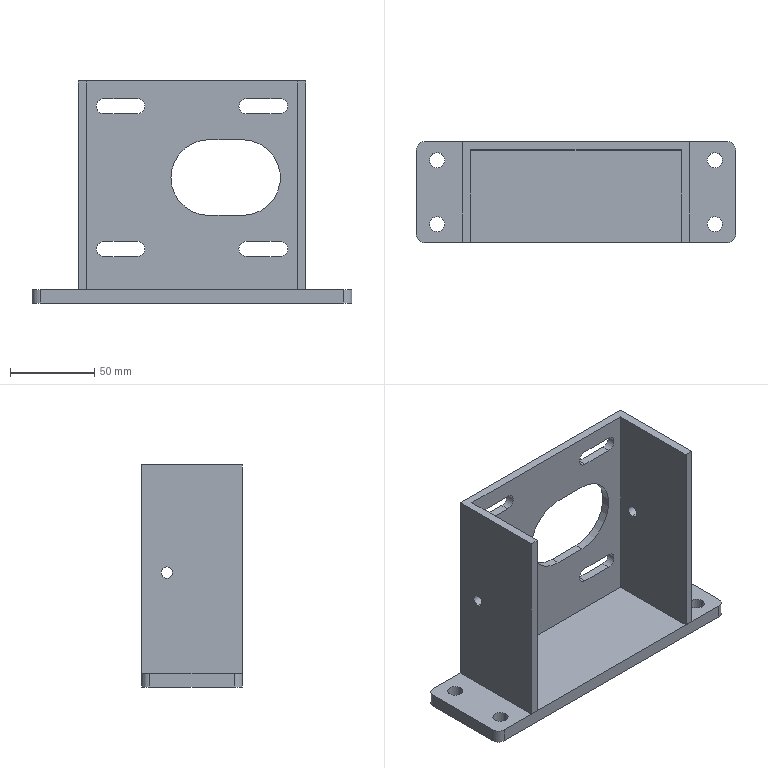Part | SolidWorks | features ICE 3, Cut 1, Extrusion 1, Fillet 1 | 2 solids | 57 faces | box 190 x 60 x 132 mm | volume 223205 mm3 | cylinder 31 | plane 26 | commonest cylinder face diameters 9 x20 6.8 x4 10 x4 45 x3